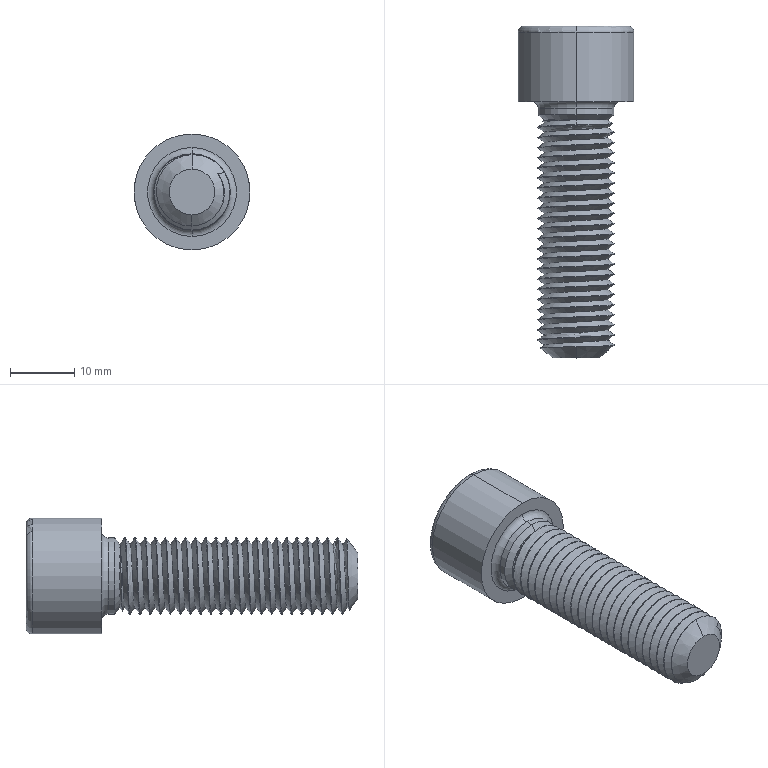Part | STEP file | Parafuso M12 - 40mm | 1 solid | 75 faces | box 18.1 x 51.8 x 18.1 mm | volume 6404 mm3 | cylinder 49 | plane 10 | cone 8 | torus 6 | spline 2 | commonest cylinder face diameters 11.9 x47 18.1 x2